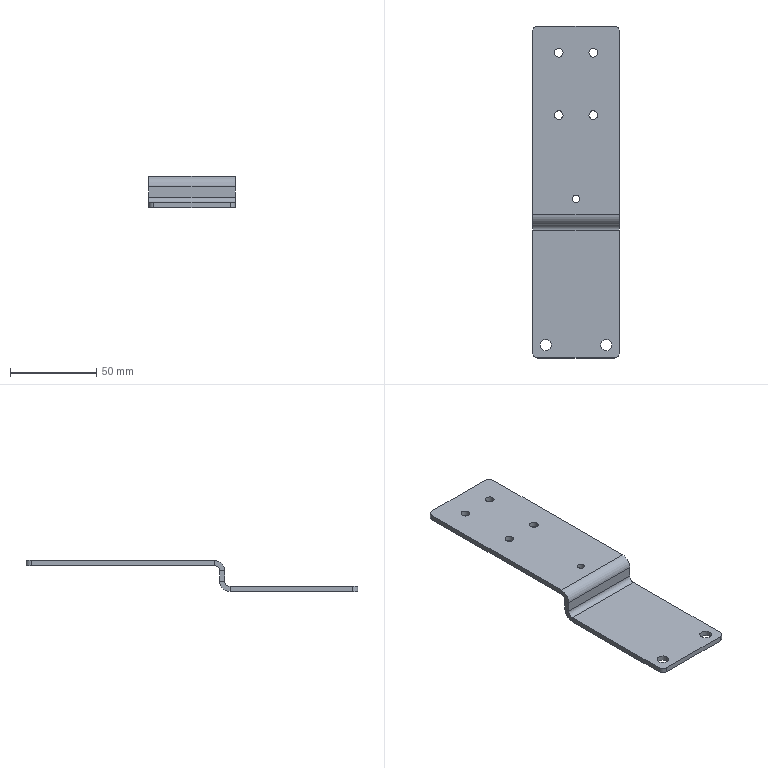Part | NX | 1 solid | 33 faces | box 50 x 192 x 18 mm | volume 29965 mm3 | plane 18 | cylinder 15 | commonest cylinder face diameters 6 x6 5 x4 6.6 x2 12 x2 4.2 x1
STEP:
#1=CARTESIAN_POINT('',(25.,40.,9.));
#2=VERTEX_POINT('',#1);
#3=CARTESIAN_POINT('',(25.,37.,9.));
#4=VERTEX_POINT('',#3);
#5=CARTESIAN_POINT('',(25.,40.,9.));
#6=DIRECTION('',(0.,-1.,0.));
#7=VECTOR('',#6,1000.);
#8=LINE('',#5,#7);
#9=EDGE_CURVE('',#2,#4,#8,.T.);
#10=ORIENTED_EDGE('',*,*,#9,.T.);
#11=CARTESIAN_POINT('',(25.,37.,3.));
#12=VERTEX_POINT('',#11);
#13=CARTESIAN_POINT('',(25.,37.,0.));
#14=DIRECTION('',(0.,0.,1.));
#15=VECTOR('',#14,1000.);
#16=LINE('',#13,#15);
#17=EDGE_CURVE('',#4,#12,#16,.F.);
#18=ORIENTED_EDGE('',*,*,#17,.T.);
#19=CARTESIAN_POINT('',(25.,40.,3.));
#20=VERTEX_POINT('',#19);
#21=CARTESIAN_POINT('',(25.,40.,3.));
#22=DIRECTION('',(0.,-1.,0.));
#23=VECTOR('',#22,1000.);
#24=LINE('',#21,#23);
#25=EDGE_CURVE('',#12,#20,#24,.F.);
#26=ORIENTED_EDGE('',*,*,#25,.T.);
#27=CARTESIAN_POINT('',(25.,40.,0.));
#28=DIRECTION('',(0.,0.,-1.));
#29=VECTOR('',#28,1000.);
#30=LINE('',#27,#29);
#31=EDGE_CURVE('',#2,#20,#30,.T.);
#32=ORIENTED_EDGE('',*,*,#31,.F.);
#33=EDGE_LOOP('',(#10,#18,#26,#32));
#34=FACE_BOUND('',#33,.T.);
#35=CARTESIAN_POINT('',(25.,40.,0.));
#36=DIRECTION('',(-1.,0.,0.));
#37=DIRECTION('',(0.,0.,1.));
#38=AXIS2_PLACEMENT_3D('',#35,#36,#37);
#39=PLANE('',#38);
#40=ADVANCED_FACE('',(#34),#39,.F.);
#41=CARTESIAN_POINT('',(-25.,40.,9.));
#42=VERTEX_POINT('',#41);
#43=CARTESIAN_POINT('',(-25.,37.,9.));
#44=VERTEX_POINT('',#43);
#45=CARTESIAN_POINT('',(-25.,40.,9.));
#46=DIRECTION('',(0.,-1.,0.));
#47=VECTOR('',#46,1000.);
#48=LINE('',#45,#47);
#49=EDGE_CURVE('',#42,#44,#48,.T.);
#50=ORIENTED_EDGE('',*,*,#49,.F.);
#51=CARTESIAN_POINT('',(-25.,40.,3.));
#52=VERTEX_POINT('',#51);
#53=CARTESIAN_POINT('',(-25.,40.,0.));
#54=DIRECTION('',(0.,0.,1.));
#55=VECTOR('',#54,1000.);
#56=LINE('',#53,#55);
#57=EDGE_CURVE('',#52,#42,#56,.T.);
#58=ORIENTED_EDGE('',*,*,#57,.F.);
#59=CARTESIAN_POINT('',(-25.,37.,3.));
#60=VERTEX_POINT('',#59);
#61=CARTESIAN_POINT('',(-25.,37.,3.));
#62=DIRECTION('',(0.,-1.,0.));
#63=VECTOR('',#62,1000.);
#64=LINE('',#61,#63);
#65=EDGE_CURVE('',#60,#52,#64,.F.);
#66=ORIENTED_EDGE('',*,*,#65,.F.);
#67=CARTESIAN_POINT('',(-25.,37.,15.));
#68=DIRECTION('',(0.,0.,-1.));
#69=VECTOR('',#68,1000.);
#70=LINE('',#67,#69);
#71=EDGE_CURVE('',#60,#44,#70,.F.);
#72=ORIENTED_EDGE('',*,*,#71,.T.);
#73=EDGE_LOOP('',(#50,#58,#66,#72));
#74=FACE_BOUND('',#73,.T.);
#75=CARTESIAN_POINT('',(-25.,40.,15.));
#76=DIRECTION('',(1.,0.,0.));
#77=DIRECTION('',(0.,0.,-1.));
#78=AXIS2_PLACEMENT_3D('',#75,#76,#77);
#79=PLANE('',#78);
#80=ADVANCED_FACE('',(#74),#79,.F.);
#81=CARTESIAN_POINT('',(25.,40.,9.));
#82=DIRECTION('',(1.,0.,0.));
#83=VECTOR('',#82,1000.);
#84=LINE('',#81,#83);
#85=EDGE_CURVE('',#2,#42,#84,.F.);
#86=ORIENTED_EDGE('',*,*,#85,.F.);
#87=ORIENTED_EDGE('',*,*,#31,.T.);
#88=CARTESIAN_POINT('',(25.,40.,3.));
#89=DIRECTION('',(-1.,0.,0.));
#90=VECTOR('',#89,1000.);
#91=LINE('',#88,#90);
#92=EDGE_CURVE('',#52,#20,#91,.F.);
#93=ORIENTED_EDGE('',*,*,#92,.F.);
#94=ORIENTED_EDGE('',*,*,#57,.T.);
#95=EDGE_LOOP('',(#86,#87,#93,#94));
#96=FACE_BOUND('',#95,.T.);
#97=CARTESIAN_POINT('',(0.,40.,0.));
#98=DIRECTION('',(0.,-1.,0.));
#99=DIRECTION('',(0.,0.,-1.));
#100=AXIS2_PLACEMENT_3D('',#97,#98,#99);
#101=PLANE('',#100);
#102=ADVANCED_FACE('',(#96),#101,.F.);
#103=ORIENTED_EDGE('',*,*,#17,.F.);
#104=CARTESIAN_POINT('',(25.,37.,9.));
#105=DIRECTION('',(1.,0.,0.));
#106=VECTOR('',#105,1000.);
#107=LINE('',#104,#106);
#108=EDGE_CURVE('',#4,#44,#107,.F.);
#109=ORIENTED_EDGE('',*,*,#108,.T.);
#110=ORIENTED_EDGE('',*,*,#71,.F.);
#111=CARTESIAN_POINT('',(25.,37.,3.));
#112=DIRECTION('',(-1.,0.,0.));
#113=VECTOR('',#112,1000.);
#114=LINE('',#111,#113);
#115=EDGE_CURVE('',#12,#60,#114,.T.);
#116=ORIENTED_EDGE('',*,*,#115,.F.);
#117=EDGE_LOOP('',(#103,#109,#110,#116));
#118=FACE_BOUND('',#117,.T.);
#119=CARTESIAN_POINT('',(0.,37.,0.));
#120=DIRECTION('',(0.,-1.,0.));
#121=DIRECTION('',(0.,0.,-1.));
#122=AXIS2_PLACEMENT_3D('',#119,#120,#121);
#123=PLANE('',#122);
#124=ADVANCED_FACE('',(#118),#123,.T.);
#125=CARTESIAN_POINT('',(-25.,34.,-3.));
#126=VERTEX_POINT('',#125);
#127=CARTESIAN_POINT('',(-25.,-37.,-3.));
#128=VERTEX_POINT('',#127);
#129=CARTESIAN_POINT('',(-25.,-40.,-3.));
#130=DIRECTION('',(0.,-1.,0.));
#131=VECTOR('',#130,1000.);
#132=LINE('',#129,#131);
#133=EDGE_CURVE('',#126,#128,#132,.T.);
#134=ORIENTED_EDGE('',*,*,#133,.T.);
#135=CARTESIAN_POINT('',(-25.,-37.,0.));
#136=VERTEX_POINT('',#135);
#137=CARTESIAN_POINT('',(-25.,-37.,-3.));
#138=DIRECTION('',(0.,0.,1.));
#139=VECTOR('',#138,1000.);
#140=LINE('',#137,#139);
#141=EDGE_CURVE('',#128,#136,#140,.T.);
#142=ORIENTED_EDGE('',*,*,#141,.T.);
#143=CARTESIAN_POINT('',(-25.,34.,0.));
#144=VERTEX_POINT('',#143);
#145=CARTESIAN_POINT('',(-25.,-40.,0.));
#146=DIRECTION('',(0.,-1.,0.));
#147=VECTOR('',#146,1000.);
#148=LINE('',#145,#147);
#149=EDGE_CURVE('',#144,#136,#148,.T.);
#150=ORIENTED_EDGE('',*,*,#149,.F.);
#151=CARTESIAN_POINT('',(-25.,34.,0.));
#152=DIRECTION('',(0.,0.,-1.));
#153=VECTOR('',#152,1000.);
#154=LINE('',#151,#153);
#155=EDGE_CURVE('',#144,#126,#154,.T.);
#156=ORIENTED_EDGE('',*,*,#155,.T.);
#157=EDGE_LOOP('',(#134,#142,#150,#156));
#158=FACE_BOUND('',#157,.T.);
#159=CARTESIAN_POINT('',(-25.,-40.,-3.));
#160=DIRECTION('',(-1.,0.,0.));
#161=DIRECTION('',(0.,0.,1.));
#162=AXIS2_PLACEMENT_3D('',#159,#160,#161);
#163=PLANE('',#162);
#164=ADVANCED_FACE('',(#158),#163,.T.);
#165=CARTESIAN_POINT('',(-14.2,-32.5,-3.));
#166=VERTEX_POINT('',#165);
#167=CARTESIAN_POINT('',(-17.5,-32.5,-3.));
#168=DIRECTION('',(0.,0.,1.));
#169=DIRECTION('',(1.,0.,0.));
#170=AXIS2_PLACEMENT_3D('',#167,#168,#169);
#171=CIRCLE('',#170,3.3);
#172=EDGE_CURVE('',#166,#166,#171,.T.);
#173=ORIENTED_EDGE('',*,*,#172,.T.);
#174=EDGE_LOOP('',(#173));
#175=FACE_BOUND('',#174,.T.);
#176=CARTESIAN_POINT('',(20.8,-32.5,-3.));
#177=VERTEX_POINT('',#176);
#178=CARTESIAN_POINT('',(17.5,-32.5,-3.));
#179=DIRECTION('',(0.,0.,1.));
#180=DIRECTION('',(1.,0.,0.));
#181=AXIS2_PLACEMENT_3D('',#178,#179,#180);
#182=CIRCLE('',#181,3.3);
#183=EDGE_CURVE('',#177,#177,#182,.T.);
#184=ORIENTED_EDGE('',*,*,#183,.T.);
#185=EDGE_LOOP('',(#184));
#186=FACE_BOUND('',#185,.T.);
#187=CARTESIAN_POINT('',(25.,-37.,-3.));
#188=VERTEX_POINT('',#187);
#189=CARTESIAN_POINT('',(25.,34.,-3.));
#190=VERTEX_POINT('',#189);
#191=CARTESIAN_POINT('',(25.,-40.,-3.));
#192=DIRECTION('',(0.,1.,0.));
#193=VECTOR('',#192,1000.);
#194=LINE('',#191,#193);
#195=EDGE_CURVE('',#188,#190,#194,.T.);
#196=ORIENTED_EDGE('',*,*,#195,.F.);
#197=CARTESIAN_POINT('',(22.,-40.,-3.));
#198=VERTEX_POINT('',#197);
#199=CARTESIAN_POINT('',(22.,-37.,-3.));
#200=DIRECTION('',(0.,0.,-1.));
#201=DIRECTION('',(-1.,0.,0.));
#202=AXIS2_PLACEMENT_3D('',#199,#200,#201);
#203=CIRCLE('',#202,3.);
#204=EDGE_CURVE('',#188,#198,#203,.T.);
#205=ORIENTED_EDGE('',*,*,#204,.T.);
#206=CARTESIAN_POINT('',(-22.,-40.,-3.));
#207=VERTEX_POINT('',#206);
#208=CARTESIAN_POINT('',(-25.,-40.,-3.));
#209=DIRECTION('',(1.,0.,0.));
#210=VECTOR('',#209,1000.);
#211=LINE('',#208,#210);
#212=EDGE_CURVE('',#207,#198,#211,.T.);
#213=ORIENTED_EDGE('',*,*,#212,.F.);
#214=CARTESIAN_POINT('',(-22.,-37.,-3.));
#215=DIRECTION('',(0.,0.,-1.));
#216=DIRECTION('',(-1.,0.,0.));
#217=AXIS2_PLACEMENT_3D('',#214,#215,#216);
#218=CIRCLE('',#217,3.);
#219=EDGE_CURVE('',#207,#128,#218,.T.);
#220=ORIENTED_EDGE('',*,*,#219,.T.);
#221=ORIENTED_EDGE('',*,*,#133,.F.);
#222=CARTESIAN_POINT('',(-25.,34.,-3.));
#223=DIRECTION('',(-1.,0.,0.));
#224=VECTOR('',#223,1000.);
#225=LINE('',#222,#224);
#226=EDGE_CURVE('',#126,#190,#225,.F.);
#227=ORIENTED_EDGE('',*,*,#226,.T.);
#228=EDGE_LOOP('',(#196,#205,#213,#220,#221,#227));
#229=FACE_BOUND('',#228,.T.);
#230=CARTESIAN_POINT('',(0.,0.,-3.));
#231=DIRECTION('',(0.,0.,-1.));
#232=DIRECTION('',(-1.,0.,0.));
#233=AXIS2_PLACEMENT_3D('',#230,#231,#232);
#234=PLANE('',#233);
#235=ADVANCED_FACE('',(#175,#186,#229),#234,.T.);
#236=CARTESIAN_POINT('',(-14.2,-32.5,0.));
#237=VERTEX_POINT('',#236);
#238=CARTESIAN_POINT('',(-17.5,-32.5,0.));
#239=DIRECTION('',(0.,0.,1.));
#240=DIRECTION('',(1.,0.,0.));
#241=AXIS2_PLACEMENT_3D('',#238,#239,#240);
#242=CIRCLE('',#241,3.3);
#243=EDGE_CURVE('',#237,#237,#242,.T.);
#244=ORIENTED_EDGE('',*,*,#243,.F.);
#245=EDGE_LOOP('',(#244));
#246=FACE_BOUND('',#245,.T.);
#247=CARTESIAN_POINT('',(20.8,-32.5,0.));
#248=VERTEX_POINT('',#247);
#249=CARTESIAN_POINT('',(17.5,-32.5,0.));
#250=DIRECTION('',(0.,0.,1.));
#251=DIRECTION('',(1.,0.,0.));
#252=AXIS2_PLACEMENT_3D('',#249,#250,#251);
#253=CIRCLE('',#252,3.3);
#254=EDGE_CURVE('',#248,#248,#253,.T.);
#255=ORIENTED_EDGE('',*,*,#254,.F.);
#256=EDGE_LOOP('',(#255));
#257=FACE_BOUND('',#256,.T.);
#258=CARTESIAN_POINT('',(-22.,-40.,0.));
#259=VERTEX_POINT('',#258);
#260=CARTESIAN_POINT('',(22.,-40.,0.));
#261=VERTEX_POINT('',#260);
#262=CARTESIAN_POINT('',(-25.,-40.,0.));
#263=DIRECTION('',(1.,0.,0.));
#264=VECTOR('',#263,1000.);
#265=LINE('',#262,#264);
#266=EDGE_CURVE('',#259,#261,#265,.T.);
#267=ORIENTED_EDGE('',*,*,#266,.T.);
#268=CARTESIAN_POINT('',(25.,-37.,0.));
#269=VERTEX_POINT('',#268);
#270=CARTESIAN_POINT('',(22.,-37.,0.));
#271=DIRECTION('',(0.,0.,-1.));
#272=DIRECTION('',(-1.,0.,0.));
#273=AXIS2_PLACEMENT_3D('',#270,#271,#272);
#274=CIRCLE('',#273,3.);
#275=EDGE_CURVE('',#261,#269,#274,.F.);
#276=ORIENTED_EDGE('',*,*,#275,.T.);
#277=CARTESIAN_POINT('',(25.,34.,0.));
#278=VERTEX_POINT('',#277);
#279=CARTESIAN_POINT('',(25.,-40.,0.));
#280=DIRECTION('',(0.,1.,0.));
#281=VECTOR('',#280,1000.);
#282=LINE('',#279,#281);
#283=EDGE_CURVE('',#269,#278,#282,.T.);
#284=ORIENTED_EDGE('',*,*,#283,.T.);
#285=CARTESIAN_POINT('',(-25.,34.,0.));
#286=DIRECTION('',(-1.,0.,0.));
#287=VECTOR('',#286,1000.);
#288=LINE('',#285,#287);
#289=EDGE_CURVE('',#144,#278,#288,.F.);
#290=ORIENTED_EDGE('',*,*,#289,.F.);
#291=ORIENTED_EDGE('',*,*,#149,.T.);
#292=CARTESIAN_POINT('',(-22.,-37.,0.));
#293=DIRECTION('',(0.,0.,-1.));
#294=DIRECTION('',(-1.,0.,0.));
#295=AXIS2_PLACEMENT_3D('',#292,#293,#294);
#296=CIRCLE('',#295,3.);
#297=EDGE_CURVE('',#136,#259,#296,.F.);
#298=ORIENTED_EDGE('',*,*,#297,.T.);
#299=EDGE_LOOP('',(#267,#276,#284,#290,#291,#298));
#300=FACE_BOUND('',#299,.T.);
#301=CARTESIAN_POINT('',(0.,0.,0.));
#302=DIRECTION('',(0.,0.,-1.));
#303=DIRECTION('',(-1.,0.,0.));
#304=AXIS2_PLACEMENT_3D('',#301,#302,#303);
#305=PLANE('',#304);
#306=ADVANCED_FACE('',(#246,#257,#300),#305,.F.);
#307=ORIENTED_EDGE('',*,*,#283,.F.);
#308=CARTESIAN_POINT('',(25.,-37.,-3.));
#309=DIRECTION('',(0.,0.,1.));
#310=VECTOR('',#309,1000.);
#311=LINE('',#308,#310);
#312=EDGE_CURVE('',#269,#188,#311,.F.);
#313=ORIENTED_EDGE('',*,*,#312,.T.);
#314=ORIENTED_EDGE('',*,*,#195,.T.);
#315=CARTESIAN_POINT('',(25.,34.,0.));
#316=DIRECTION('',(0.,0.,-1.));
#317=VECTOR('',#316,1000.);
#318=LINE('',#315,#317);
#319=EDGE_CURVE('',#278,#190,#318,.T.);
#320=ORIENTED_EDGE('',*,*,#319,.F.);
#321=EDGE_LOOP('',(#307,#313,#314,#320));
#322=FACE_BOUND('',#321,.T.);
#323=CARTESIAN_POINT('',(25.,-40.,-3.));
#324=DIRECTION('',(1.,0.,0.));
#325=DIRECTION('',(0.,0.,-1.));
#326=AXIS2_PLACEMENT_3D('',#323,#324,#325);
#327=PLANE('',#326);
#328=ADVANCED_FACE('',(#322),#327,.T.);
#329=ORIENTED_EDGE('',*,*,#212,.T.);
#330=CARTESIAN_POINT('',(22.,-40.,-3.));
#331=DIRECTION('',(0.,0.,1.));
#332=VECTOR('',#331,1000.);
#333=LINE('',#330,#332);
#334=EDGE_CURVE('',#198,#261,#333,.T.);
#335=ORIENTED_EDGE('',*,*,#334,.T.);
#336=ORIENTED_EDGE('',*,*,#266,.F.);
#337=CARTESIAN_POINT('',(-22.,-40.,-3.));
#338=DIRECTION('',(0.,0.,1.));
#339=VECTOR('',#338,1000.);
#340=LINE('',#337,#339);
#341=EDGE_CURVE('',#259,#207,#340,.F.);
#342=ORIENTED_EDGE('',*,*,#341,.T.);
#343=EDGE_LOOP('',(#329,#335,#336,#342));
#344=FACE_BOUND('',#343,.T.);
#345=CARTESIAN_POINT('',(-25.,-40.,-3.));
#346=DIRECTION('',(0.,-1.,0.));
#347=DIRECTION('',(0.,0.,-1.));
#348=AXIS2_PLACEMENT_3D('',#345,#346,#347);
#349=PLANE('',#348);
#350=ADVANCED_FACE('',(#344),#349,.T.);
#351=ORIENTED_EDGE('',*,*,#25,.F.);
#352=CARTESIAN_POINT('',(25.,34.,3.));
#353=DIRECTION('',(-1.,0.,0.));
#354=DIRECTION('',(0.,0.,1.));
#355=AXIS2_PLACEMENT_3D('',#352,#353,#354);
#356=CIRCLE('',#355,3.);
#357=EDGE_CURVE('',#278,#12,#356,.F.);
#358=ORIENTED_EDGE('',*,*,#357,.F.);
#359=ORIENTED_EDGE('',*,*,#319,.T.);
#360=CARTESIAN_POINT('',(25.,34.,3.));
#361=DIRECTION('',(-1.,0.,0.));
#362=DIRECTION('',(0.,0.,1.));
#363=AXIS2_PLACEMENT_3D('',#360,#361,#362);
#364=CIRCLE('',#363,6.);
#365=EDGE_CURVE('',#190,#20,#364,.F.);
#366=ORIENTED_EDGE('',*,*,#365,.T.);
#367=EDGE_LOOP('',(#351,#358,#359,#366));
#368=FACE_BOUND('',#367,.T.);
#369=CARTESIAN_POINT('',(25.,34.,3.));
#370=DIRECTION('',(1.,0.,0.));
#371=DIRECTION('',(0.,0.,-1.));
#372=AXIS2_PLACEMENT_3D('',#369,#370,#371);
#373=PLANE('',#372);
#374=ADVANCED_FACE('',(#368),#373,.T.);
#375=CARTESIAN_POINT('',(-25.,34.,3.));
#376=DIRECTION('',(-1.,0.,0.));
#377=DIRECTION('',(0.,0.,1.));
#378=AXIS2_PLACEMENT_3D('',#375,#376,#377);
#379=CIRCLE('',#378,3.);
#380=EDGE_CURVE('',#60,#144,#379,.T.);
#381=ORIENTED_EDGE('',*,*,#380,.F.);
#382=ORIENTED_EDGE('',*,*,#65,.T.);
#383=CARTESIAN_POINT('',(-25.,34.,3.));
#384=DIRECTION('',(-1.,0.,0.));
#385=DIRECTION('',(0.,0.,1.));
#386=AXIS2_PLACEMENT_3D('',#383,#384,#385);
#387=CIRCLE('',#386,6.);
#388=EDGE_CURVE('',#52,#126,#387,.T.);
#389=ORIENTED_EDGE('',*,*,#388,.T.);
#390=ORIENTED_EDGE('',*,*,#155,.F.);
#391=EDGE_LOOP('',(#381,#382,#389,#390));
#392=FACE_BOUND('',#391,.T.);
#393=CARTESIAN_POINT('',(-25.,34.,3.));
#394=DIRECTION('',(1.,0.,0.));
#395=DIRECTION('',(0.,0.,-1.));
#396=AXIS2_PLACEMENT_3D('',#393,#394,#395);
#397=PLANE('',#396);
#398=ADVANCED_FACE('',(#392),#397,.F.);
#399=ORIENTED_EDGE('',*,*,#226,.F.);
#400=ORIENTED_EDGE('',*,*,#388,.F.);
#401=ORIENTED_EDGE('',*,*,#92,.T.);
#402=ORIENTED_EDGE('',*,*,#365,.F.);
#403=EDGE_LOOP('',(#399,#400,#401,#402));
#404=FACE_BOUND('',#403,.T.);
#405=CARTESIAN_POINT('',(-25.,34.,3.));
#406=DIRECTION('',(-1.,0.,0.));
#407=DIRECTION('',(0.,1.,0.));
#408=AXIS2_PLACEMENT_3D('',#405,#406,#407);
#409=CYLINDRICAL_SURFACE('',#408,6.);
#410=ADVANCED_FACE('',(#404),#409,.T.);
#411=ORIENTED_EDGE('',*,*,#289,.T.);
#412=ORIENTED_EDGE('',*,*,#357,.T.);
#413=ORIENTED_EDGE('',*,*,#115,.T.);
#414=ORIENTED_EDGE('',*,*,#380,.T.);
#415=EDGE_LOOP('',(#411,#412,#413,#414));
#416=FACE_BOUND('',#415,.T.);
#417=CARTESIAN_POINT('',(-25.,34.,3.));
#418=DIRECTION('',(-1.,0.,0.));
#419=DIRECTION('',(0.,1.,0.));
#420=AXIS2_PLACEMENT_3D('',#417,#418,#419);
#421=CYLINDRICAL_SURFACE('',#420,3.);
#422=ADVANCED_FACE('',(#416),#421,.F.);
#423=CARTESIAN_POINT('',(-25.,43.,12.));
#424=VERTEX_POINT('',#423);
#425=CARTESIAN_POINT('',(-25.,43.,15.));
#426=VERTEX_POINT('',#425);
#427=CARTESIAN_POINT('',(-25.,43.,15.));
#428=DIRECTION('',(0.,0.,-1.));
#429=VECTOR('',#428,1000.);
#430=LINE('',#427,#429);
#431=EDGE_CURVE('',#424,#426,#430,.F.);
#432=ORIENTED_EDGE('',*,*,#431,.F.);
#433=CARTESIAN_POINT('',(-25.,43.,9.));
#434=DIRECTION('',(1.,0.,0.));
#435=DIRECTION('',(0.,0.,-1.));
#436=AXIS2_PLACEMENT_3D('',#433,#434,#435);
#437=CIRCLE('',#436,3.);
#438=EDGE_CURVE('',#42,#424,#437,.F.);
#439=ORIENTED_EDGE('',*,*,#438,.F.);
#440=ORIENTED_EDGE('',*,*,#49,.T.);
#441=CARTESIAN_POINT('',(-25.,43.,9.));
#442=DIRECTION('',(1.,0.,0.));
#443=DIRECTION('',(0.,0.,-1.));
#444=AXIS2_PLACEMENT_3D('',#441,#442,#443);
#445=CIRCLE('',#444,6.);
#446=EDGE_CURVE('',#44,#426,#445,.F.);
#447=ORIENTED_EDGE('',*,*,#446,.T.);
#448=EDGE_LOOP('',(#432,#439,#440,#447));
#449=FACE_BOUND('',#448,.T.);
#450=CARTESIAN_POINT('',(-25.,43.,9.));
#451=DIRECTION('',(-1.,0.,0.));
#452=DIRECTION('',(0.,0.,1.));
#453=AXIS2_PLACEMENT_3D('',#450,#451,#452);
#454=PLANE('',#453);
#455=ADVANCED_FACE('',(#449),#454,.T.);
#456=CARTESIAN_POINT('',(25.,43.,12.));
#457=VERTEX_POINT('',#456);
#458=CARTESIAN_POINT('',(25.,43.,9.));
#459=DIRECTION('',(1.,0.,0.));
#460=DIRECTION('',(0.,0.,-1.));
#461=AXIS2_PLACEMENT_3D('',#458,#459,#460);
#462=CIRCLE('',#461,3.);
#463=EDGE_CURVE('',#457,#2,#462,.T.);
#464=ORIENTED_EDGE('',*,*,#463,.F.);
#465=CARTESIAN_POINT('',(25.,43.,15.));
#466=VERTEX_POINT('',#465);
#467=CARTESIAN_POINT('',(25.,43.,12.));
#468=DIRECTION('',(0.,0.,-1.));
#469=VECTOR('',#468,1000.);
#470=LINE('',#467,#469);
#471=EDGE_CURVE('',#457,#466,#470,.F.);
#472=ORIENTED_EDGE('',*,*,#471,.T.);
#473=CARTESIAN_POINT('',(25.,43.,9.));
#474=DIRECTION('',(1.,0.,0.));
#475=DIRECTION('',(0.,0.,-1.));
#476=AXIS2_PLACEMENT_3D('',#473,#474,#475);
#477=CIRCLE('',#476,6.);
#478=EDGE_CURVE('',#466,#4,#477,.T.);
#479=ORIENTED_EDGE('',*,*,#478,.T.);
#480=ORIENTED_EDGE('',*,*,#9,.F.);
#481=EDGE_LOOP('',(#464,#472,#479,#480));
#482=FACE_BOUND('',#481,.T.);
#483=CARTESIAN_POINT('',(25.,43.,9.));
#484=DIRECTION('',(-1.,0.,0.));
#485=DIRECTION('',(0.,0.,1.));
#486=AXIS2_PLACEMENT_3D('',#483,#484,#485);
#487=PLANE('',#486);
#488=ADVANCED_FACE('',(#482),#487,.F.);
#489=ORIENTED_EDGE('',*,*,#108,.F.);
#490=ORIENTED_EDGE('',*,*,#478,.F.);
#491=CARTESIAN_POINT('',(-25.,43.,15.));
#492=DIRECTION('',(1.,0.,0.));
#493=VECTOR('',#492,1000.);
#494=LINE('',#491,#493);
#495=EDGE_CURVE('',#466,#426,#494,.F.);
#496=ORIENTED_EDGE('',*,*,#495,.T.);
#497=ORIENTED_EDGE('',*,*,#446,.F.);
#498=EDGE_LOOP('',(#489,#490,#496,#497));
#499=FACE_BOUND('',#498,.T.);
#500=CARTESIAN_POINT('',(25.,43.,9.));
#501=DIRECTION('',(1.,0.,0.));
#502=DIRECTION('',(0.,0.,1.));
#503=AXIS2_PLACEMENT_3D('',#500,#501,#502);
#504=CYLINDRICAL_SURFACE('',#503,6.);
#505=ADVANCED_FACE('',(#499),#504,.T.);
#506=ORIENTED_EDGE('',*,*,#85,.T.);
#507=ORIENTED_EDGE('',*,*,#438,.T.);
#508=CARTESIAN_POINT('',(-25.,43.,12.));
#509=DIRECTION('',(1.,0.,0.));
#510=VECTOR('',#509,1000.);
#511=LINE('',#508,#510);
#512=EDGE_CURVE('',#424,#457,#511,.T.);
#513=ORIENTED_EDGE('',*,*,#512,.T.);
#514=ORIENTED_EDGE('',*,*,#463,.T.);
#515=EDGE_LOOP('',(#506,#507,#513,#514));
#516=FACE_BOUND('',#515,.T.);
#517=CARTESIAN_POINT('',(25.,43.,9.));
#518=DIRECTION('',(1.,0.,0.));
#519=DIRECTION('',(0.,0.,1.));
#520=AXIS2_PLACEMENT_3D('',#517,#518,#519);
#521=CYLINDRICAL_SURFACE('',#520,3.);
#522=ADVANCED_FACE('',(#516),#521,.F.);
#523=CARTESIAN_POINT('',(-25.,149.,15.));
#524=VERTEX_POINT('',#523);
#525=CARTESIAN_POINT('',(-25.,0.,15.));
#526=DIRECTION('',(0.,-1.,0.));
#527=VECTOR('',#526,1000.);
#528=LINE('',#525,#527);
#529=EDGE_CURVE('',#524,#426,#528,.T.);
#530=ORIENTED_EDGE('',*,*,#529,.F.);
#531=CARTESIAN_POINT('',(-25.,149.,12.));
#532=VERTEX_POINT('',#531);
#533=CARTESIAN_POINT('',(-25.,149.,15.));
#534=DIRECTION('',(0.,0.,-1.));
#535=VECTOR('',#534,1000.);
#536=LINE('',#533,#535);
#537=EDGE_CURVE('',#524,#532,#536,.T.);
#538=ORIENTED_EDGE('',*,*,#537,.T.);
#539=CARTESIAN_POINT('',(-25.,40.,12.));
#540=DIRECTION('',(0.,1.,0.));
#541=VECTOR('',#540,1000.);
#542=LINE('',#539,#541);
#543=EDGE_CURVE('',#532,#424,#542,.F.);
#544=ORIENTED_EDGE('',*,*,#543,.T.);
#545=ORIENTED_EDGE('',*,*,#431,.T.);
#546=EDGE_LOOP('',(#530,#538,#544,#545));
#547=FACE_BOUND('',#546,.T.);
#548=CARTESIAN_POINT('',(-25.,40.,15.));
#549=DIRECTION('',(1.,0.,0.));
#550=DIRECTION('',(0.,0.,-1.));
#551=AXIS2_PLACEMENT_3D('',#548,#549,#550);
#552=PLANE('',#551);
#553=ADVANCED_FACE('',(#547),#552,.F.);
#554=CARTESIAN_POINT('',(25.,149.,12.));
#555=VERTEX_POINT('',#554);
#556=CARTESIAN_POINT('',(25.,152.,12.));
#557=DIRECTION('',(0.,-1.,0.));
#558=VECTOR('',#557,1000.);
#559=LINE('',#556,#558);
#560=EDGE_CURVE('',#457,#555,#559,.F.);
#561=ORIENTED_EDGE('',*,*,#560,.T.);
#562=CARTESIAN_POINT('',(25.,149.,15.));
#563=VERTEX_POINT('',#562);
#564=CARTESIAN_POINT('',(25.,149.,15.));
#565=DIRECTION('',(0.,0.,-1.));
#566=VECTOR('',#565,1000.);
#567=LINE('',#564,#566);
#568=EDGE_CURVE('',#555,#563,#567,.F.);
#569=ORIENTED_EDGE('',*,*,#568,.T.);
#570=CARTESIAN_POINT('',(25.,0.,15.));
#571=DIRECTION('',(0.,1.,0.));
#572=VECTOR('',#571,1000.);
#573=LINE('',#570,#572);
#574=EDGE_CURVE('',#466,#563,#573,.T.);
#575=ORIENTED_EDGE('',*,*,#574,.F.);
#576=ORIENTED_EDGE('',*,*,#471,.F.);
#577=EDGE_LOOP('',(#561,#569,#575,#576));
#578=FACE_BOUND('',#577,.T.);
#579=CARTESIAN_POINT('',(25.,152.,15.));
#580=DIRECTION('',(-1.,0.,0.));
#581=DIRECTION('',(0.,-1.,0.));
#582=AXIS2_PLACEMENT_3D('',#579,#580,#581);
#583=PLANE('',#582);
#584=ADVANCED_FACE('',(#578),#583,.F.);
#585=CARTESIAN_POINT('',(2.1,52.,15.));
#586=VERTEX_POINT('',#585);
#587=CARTESIAN_POINT('',(0.,52.,15.));
#588=DIRECTION('',(0.,0.,1.));
#589=DIRECTION('',(1.,0.,0.));
#590=AXIS2_PLACEMENT_3D('',#587,#588,#589);
#591=CIRCLE('',#590,2.1);
#592=EDGE_CURVE('',#586,#586,#591,.T.);
#593=ORIENTED_EDGE('',*,*,#592,.F.);
#594=EDGE_LOOP('',(#593));
#595=FACE_BOUND('',#594,.T.);
#596=CARTESIAN_POINT('',(12.5,136.5,15.));
#597=VERTEX_POINT('',#596);
#598=CARTESIAN_POINT('',(10.,136.5,15.));
#599=DIRECTION('',(0.,0.,1.));
#600=DIRECTION('',(1.,0.,0.));
#601=AXIS2_PLACEMENT_3D('',#598,#599,#600);
#602=CIRCLE('',#601,2.5);
#603=EDGE_CURVE('',#597,#597,#602,.T.);
#604=ORIENTED_EDGE('',*,*,#603,.F.);
#605=EDGE_LOOP('',(#604));
#606=FACE_BOUND('',#605,.T.);
#607=CARTESIAN_POINT('',(-7.5,136.5,15.));
#608=VERTEX_POINT('',#607);
#609=CARTESIAN_POINT('',(-10.,136.5,15.));
#610=DIRECTION('',(0.,0.,1.));
#611=DIRECTION('',(1.,0.,0.));
#612=AXIS2_PLACEMENT_3D('',#609,#610,#611);
#613=CIRCLE('',#612,2.5);
#614=EDGE_CURVE('',#608,#608,#613,.T.);
#615=ORIENTED_EDGE('',*,*,#614,.F.);
#616=EDGE_LOOP('',(#615));
#617=FACE_BOUND('',#616,.T.);
#618=CARTESIAN_POINT('',(-7.5,100.5,15.));
#619=VERTEX_POINT('',#618);
#620=CARTESIAN_POINT('',(-10.,100.5,15.));
#621=DIRECTION('',(0.,0.,1.));
#622=DIRECTION('',(1.,0.,0.));
#623=AXIS2_PLACEMENT_3D('',#620,#621,#622);
#624=CIRCLE('',#623,2.5);
#625=EDGE_CURVE('',#619,#619,#624,.T.);
#626=ORIENTED_EDGE('',*,*,#625,.F.);
#627=EDGE_LOOP('',(#626));
#628=FACE_BOUND('',#627,.T.);
#629=CARTESIAN_POINT('',(12.5,100.5,15.));
#630=VERTEX_POINT('',#629);
#631=CARTESIAN_POINT('',(10.,100.5,15.));
#632=DIRECTION('',(0.,0.,1.));
#633=DIRECTION('',(1.,0.,0.));
#634=AXIS2_PLACEMENT_3D('',#631,#632,#633);
#635=CIRCLE('',#634,2.5);
#636=EDGE_CURVE('',#630,#630,#635,.T.);
#637=ORIENTED_EDGE('',*,*,#636,.F.);
#638=EDGE_LOOP('',(#637));
#639=FACE_BOUND('',#638,.T.);
#640=ORIENTED_EDGE('',*,*,#574,.T.);
#641=CARTESIAN_POINT('',(22.,152.,15.));
#642=VERTEX_POINT('',#641);
#643=CARTESIAN_POINT('',(22.,149.,15.));
#644=DIRECTION('',(0.,0.,-1.));
#645=DIRECTION('',(-1.,0.,0.));
#646=AXIS2_PLACEMENT_3D('',#643,#644,#645);
#647=CIRCLE('',#646,3.);
#648=EDGE_CURVE('',#563,#642,#647,.F.);
#649=ORIENTED_EDGE('',*,*,#648,.T.);
#650=CARTESIAN_POINT('',(-22.,152.,15.));
#651=VERTEX_POINT('',#650);
#652=CARTESIAN_POINT('',(0.,152.,15.));
#653=DIRECTION('',(-1.,0.,0.));
#654=VECTOR('',#653,1000.);
#655=LINE('',#652,#654);
#656=EDGE_CURVE('',#642,#651,#655,.T.);
#657=ORIENTED_EDGE('',*,*,#656,.T.);
#658=CARTESIAN_POINT('',(-22.,149.,15.));
#659=DIRECTION('',(0.,0.,-1.));
#660=DIRECTION('',(-1.,0.,0.));
#661=AXIS2_PLACEMENT_3D('',#658,#659,#660);
#662=CIRCLE('',#661,3.);
#663=EDGE_CURVE('',#651,#524,#662,.F.);
#664=ORIENTED_EDGE('',*,*,#663,.T.);
#665=ORIENTED_EDGE('',*,*,#529,.T.);
#666=ORIENTED_EDGE('',*,*,#495,.F.);
#667=EDGE_LOOP('',(#640,#649,#657,#664,#665,#666));
#668=FACE_BOUND('',#667,.T.);
#669=CARTESIAN_POINT('',(0.,0.,15.));
#670=DIRECTION('',(0.,0.,-1.));
#671=DIRECTION('',(-1.,0.,0.));
#672=AXIS2_PLACEMENT_3D('',#669,#670,#671);
#673=PLANE('',#672);
#674=ADVANCED_FACE('',(#595,#606,#617,#628,#639,#668),#673,.F.);
#675=CARTESIAN_POINT('',(-2.1,52.,12.));
#676=VERTEX_POINT('',#675);
#677=CARTESIAN_POINT('',(0.,52.,12.));
#678=DIRECTION('',(0.,0.,-1.));
#679=DIRECTION('',(-1.,0.,0.));
#680=AXIS2_PLACEMENT_3D('',#677,#678,#679);
#681=CIRCLE('',#680,2.1);
#682=EDGE_CURVE('',#676,#676,#681,.T.);
#683=ORIENTED_EDGE('',*,*,#682,.F.);
#684=EDGE_LOOP('',(#683));
#685=FACE_BOUND('',#684,.T.);
#686=CARTESIAN_POINT('',(7.5,136.5,12.));
#687=VERTEX_POINT('',#686);
#688=CARTESIAN_POINT('',(10.,136.5,12.));
#689=DIRECTION('',(0.,0.,-1.));
#690=DIRECTION('',(-1.,0.,0.));
#691=AXIS2_PLACEMENT_3D('',#688,#689,#690);
#692=CIRCLE('',#691,2.5);
#693=EDGE_CURVE('',#687,#687,#692,.T.);
#694=ORIENTED_EDGE('',*,*,#693,.F.);
#695=EDGE_LOOP('',(#694));
#696=FACE_BOUND('',#695,.T.);
#697=CARTESIAN_POINT('',(-12.5,136.5,12.));
#698=VERTEX_POINT('',#697);
#699=CARTESIAN_POINT('',(-10.,136.5,12.));
#700=DIRECTION('',(0.,0.,-1.));
#701=DIRECTION('',(-1.,0.,0.));
#702=AXIS2_PLACEMENT_3D('',#699,#700,#701);
#703=CIRCLE('',#702,2.5);
#704=EDGE_CURVE('',#698,#698,#703,.T.);
#705=ORIENTED_EDGE('',*,*,#704,.F.);
#706=EDGE_LOOP('',(#705));
#707=FACE_BOUND('',#706,.T.);
#708=CARTESIAN_POINT('',(-12.5,100.5,12.));
#709=VERTEX_POINT('',#708);
#710=CARTESIAN_POINT('',(-10.,100.5,12.));
#711=DIRECTION('',(0.,0.,-1.));
#712=DIRECTION('',(-1.,0.,0.));
#713=AXIS2_PLACEMENT_3D('',#710,#711,#712);
#714=CIRCLE('',#713,2.5);
#715=EDGE_CURVE('',#709,#709,#714,.T.);
#716=ORIENTED_EDGE('',*,*,#715,.F.);
#717=EDGE_LOOP('',(#716));
#718=FACE_BOUND('',#717,.T.);
#719=CARTESIAN_POINT('',(7.5,100.5,12.));
#720=VERTEX_POINT('',#719);
#721=CARTESIAN_POINT('',(10.,100.5,12.));
#722=DIRECTION('',(0.,0.,-1.));
#723=DIRECTION('',(-1.,0.,0.));
#724=AXIS2_PLACEMENT_3D('',#721,#722,#723);
#725=CIRCLE('',#724,2.5);
#726=EDGE_CURVE('',#720,#720,#725,.T.);
#727=ORIENTED_EDGE('',*,*,#726,.F.);
#728=EDGE_LOOP('',(#727));
#729=FACE_BOUND('',#728,.T.);
#730=CARTESIAN_POINT('',(22.,152.,12.));
#731=VERTEX_POINT('',#730);
#732=CARTESIAN_POINT('',(-22.,152.,12.));
#733=VERTEX_POINT('',#732);
#734=CARTESIAN_POINT('',(-25.,152.,12.));
#735=DIRECTION('',(1.,0.,0.));
#736=VECTOR('',#735,1000.);
#737=LINE('',#734,#736);
#738=EDGE_CURVE('',#731,#733,#737,.F.);
#739=ORIENTED_EDGE('',*,*,#738,.F.);
#740=CARTESIAN_POINT('',(22.,149.,12.));
#741=DIRECTION('',(0.,0.,-1.));
#742=DIRECTION('',(-1.,0.,0.));
#743=AXIS2_PLACEMENT_3D('',#740,#741,#742);
#744=CIRCLE('',#743,3.);
#745=EDGE_CURVE('',#731,#555,#744,.T.);
#746=ORIENTED_EDGE('',*,*,#745,.T.);
#747=ORIENTED_EDGE('',*,*,#560,.F.);
#748=ORIENTED_EDGE('',*,*,#512,.F.);
#749=ORIENTED_EDGE('',*,*,#543,.F.);
#750=CARTESIAN_POINT('',(-22.,149.,12.));
#751=DIRECTION('',(0.,0.,-1.));
#752=DIRECTION('',(-1.,0.,0.));
#753=AXIS2_PLACEMENT_3D('',#750,#751,#752);
#754=CIRCLE('',#753,3.);
#755=EDGE_CURVE('',#532,#733,#754,.T.);
#756=ORIENTED_EDGE('',*,*,#755,.T.);
#757=EDGE_LOOP('',(#739,#746,#747,#748,#749,#756));
#758=FACE_BOUND('',#757,.T.);
#759=CARTESIAN_POINT('',(0.,0.,12.));
#760=DIRECTION('',(0.,0.,-1.));
#761=DIRECTION('',(-1.,0.,0.));
#762=AXIS2_PLACEMENT_3D('',#759,#760,#761);
#763=PLANE('',#762);
#764=ADVANCED_FACE('',(#685,#696,#707,#718,#729,#758),#763,.T.);
#765=ORIENTED_EDGE('',*,*,#656,.F.);
#766=CARTESIAN_POINT('',(22.,152.,15.));
#767=DIRECTION('',(0.,0.,-1.));
#768=VECTOR('',#767,1000.);
#769=LINE('',#766,#768);
#770=EDGE_CURVE('',#642,#731,#769,.T.);
#771=ORIENTED_EDGE('',*,*,#770,.T.);
#772=ORIENTED_EDGE('',*,*,#738,.T.);
#773=CARTESIAN_POINT('',(-22.,152.,15.));
#774=DIRECTION('',(0.,0.,-1.));
#775=VECTOR('',#774,1000.);
#776=LINE('',#773,#775);
#777=EDGE_CURVE('',#733,#651,#776,.F.);
#778=ORIENTED_EDGE('',*,*,#777,.T.);
#779=EDGE_LOOP('',(#765,#771,#772,#778));
#780=FACE_BOUND('',#779,.T.);
#781=CARTESIAN_POINT('',(-25.,152.,15.));
#782=DIRECTION('',(0.,-1.,0.));
#783=DIRECTION('',(0.,0.,-1.));
#784=AXIS2_PLACEMENT_3D('',#781,#782,#783);
#785=PLANE('',#784);
#786=ADVANCED_FACE('',(#780),#785,.F.);
#787=ORIENTED_EDGE('',*,*,#183,.F.);
#788=EDGE_LOOP('',(#787));
#789=FACE_BOUND('',#788,.T.);
#790=ORIENTED_EDGE('',*,*,#254,.T.);
#791=EDGE_LOOP('',(#790));
#792=FACE_BOUND('',#791,.T.);
#793=CARTESIAN_POINT('',(17.5,-32.5,0.));
#794=DIRECTION('',(0.,0.,1.));
#795=DIRECTION('',(1.,0.,0.));
#796=AXIS2_PLACEMENT_3D('',#793,#794,#795);
#797=CYLINDRICAL_SURFACE('',#796,3.3);
#798=ADVANCED_FACE('',(#789,#792),#797,.F.);
#799=ORIENTED_EDGE('',*,*,#172,.F.);
#800=EDGE_LOOP('',(#799));
#801=FACE_BOUND('',#800,.T.);
#802=ORIENTED_EDGE('',*,*,#243,.T.);
#803=EDGE_LOOP('',(#802));
#804=FACE_BOUND('',#803,.T.);
#805=CARTESIAN_POINT('',(-17.5,-32.5,0.));
#806=DIRECTION('',(0.,0.,1.));
#807=DIRECTION('',(1.,0.,0.));
#808=AXIS2_PLACEMENT_3D('',#805,#806,#807);
#809=CYLINDRICAL_SURFACE('',#808,3.3);
#810=ADVANCED_FACE('',(#801,#804),#809,.F.);
#811=ORIENTED_EDGE('',*,*,#726,.T.);
#812=EDGE_LOOP('',(#811));
#813=FACE_BOUND('',#812,.T.);
#814=ORIENTED_EDGE('',*,*,#636,.T.);
#815=EDGE_LOOP('',(#814));
#816=FACE_BOUND('',#815,.T.);
#817=CARTESIAN_POINT('',(10.,100.5,15.));
#818=DIRECTION('',(0.,0.,1.));
#819=DIRECTION('',(1.,0.,0.));
#820=AXIS2_PLACEMENT_3D('',#817,#818,#819);
#821=CYLINDRICAL_SURFACE('',#820,2.5);
#822=ADVANCED_FACE('',(#813,#816),#821,.F.);
#823=ORIENTED_EDGE('',*,*,#715,.T.);
#824=EDGE_LOOP('',(#823));
#825=FACE_BOUND('',#824,.T.);
#826=ORIENTED_EDGE('',*,*,#625,.T.);
#827=EDGE_LOOP('',(#826));
#828=FACE_BOUND('',#827,.T.);
#829=CARTESIAN_POINT('',(-10.,100.5,15.));
#830=DIRECTION('',(0.,0.,1.));
#831=DIRECTION('',(1.,0.,0.));
#832=AXIS2_PLACEMENT_3D('',#829,#830,#831);
#833=CYLINDRICAL_SURFACE('',#832,2.5);
#834=ADVANCED_FACE('',(#825,#828),#833,.F.);
#835=ORIENTED_EDGE('',*,*,#704,.T.);
#836=EDGE_LOOP('',(#835));
#837=FACE_BOUND('',#836,.T.);
#838=ORIENTED_EDGE('',*,*,#614,.T.);
#839=EDGE_LOOP('',(#838));
#840=FACE_BOUND('',#839,.T.);
#841=CARTESIAN_POINT('',(-10.,136.5,15.));
#842=DIRECTION('',(0.,0.,1.));
#843=DIRECTION('',(1.,0.,0.));
#844=AXIS2_PLACEMENT_3D('',#841,#842,#843);
#845=CYLINDRICAL_SURFACE('',#844,2.5);
#846=ADVANCED_FACE('',(#837,#840),#845,.F.);
#847=ORIENTED_EDGE('',*,*,#693,.T.);
#848=EDGE_LOOP('',(#847));
#849=FACE_BOUND('',#848,.T.);
#850=ORIENTED_EDGE('',*,*,#603,.T.);
#851=EDGE_LOOP('',(#850));
#852=FACE_BOUND('',#851,.T.);
#853=CARTESIAN_POINT('',(10.,136.5,15.));
#854=DIRECTION('',(0.,0.,1.));
#855=DIRECTION('',(1.,0.,0.));
#856=AXIS2_PLACEMENT_3D('',#853,#854,#855);
#857=CYLINDRICAL_SURFACE('',#856,2.5);
#858=ADVANCED_FACE('',(#849,#852),#857,.F.);
#859=ORIENTED_EDGE('',*,*,#682,.T.);
#860=EDGE_LOOP('',(#859));
#861=FACE_BOUND('',#860,.T.);
#862=ORIENTED_EDGE('',*,*,#592,.T.);
#863=EDGE_LOOP('',(#862));
#864=FACE_BOUND('',#863,.T.);
#865=CARTESIAN_POINT('',(0.,52.,15.));
#866=DIRECTION('',(0.,0.,1.));
#867=DIRECTION('',(1.,0.,0.));
#868=AXIS2_PLACEMENT_3D('',#865,#866,#867);
#869=CYLINDRICAL_SURFACE('',#868,2.1);
#870=ADVANCED_FACE('',(#861,#864),#869,.F.);
#871=ORIENTED_EDGE('',*,*,#648,.F.);
#872=ORIENTED_EDGE('',*,*,#568,.F.);
#873=ORIENTED_EDGE('',*,*,#745,.F.);
#874=ORIENTED_EDGE('',*,*,#770,.F.);
#875=EDGE_LOOP('',(#871,#872,#873,#874));
#876=FACE_BOUND('',#875,.T.);
#877=CARTESIAN_POINT('',(22.,149.,15.));
#878=DIRECTION('',(0.,0.,-1.));
#879=DIRECTION('',(-1.,0.,0.));
#880=AXIS2_PLACEMENT_3D('',#877,#878,#879);
#881=CYLINDRICAL_SURFACE('',#880,3.);
#882=ADVANCED_FACE('',(#876),#881,.T.);
#883=ORIENTED_EDGE('',*,*,#204,.F.);
#884=ORIENTED_EDGE('',*,*,#312,.F.);
#885=ORIENTED_EDGE('',*,*,#275,.F.);
#886=ORIENTED_EDGE('',*,*,#334,.F.);
#887=EDGE_LOOP('',(#883,#884,#885,#886));
#888=FACE_BOUND('',#887,.T.);
#889=CARTESIAN_POINT('',(22.,-37.,-3.));
#890=DIRECTION('',(0.,0.,1.));
#891=DIRECTION('',(1.,0.,0.));
#892=AXIS2_PLACEMENT_3D('',#889,#890,#891);
#893=CYLINDRICAL_SURFACE('',#892,3.);
#894=ADVANCED_FACE('',(#888),#893,.T.);
#895=ORIENTED_EDGE('',*,*,#219,.F.);
#896=ORIENTED_EDGE('',*,*,#341,.F.);
#897=ORIENTED_EDGE('',*,*,#297,.F.);
#898=ORIENTED_EDGE('',*,*,#141,.F.);
#899=EDGE_LOOP('',(#895,#896,#897,#898));
#900=FACE_BOUND('',#899,.T.);
#901=CARTESIAN_POINT('',(-22.,-37.,-3.));
#902=DIRECTION('',(0.,0.,1.));
#903=DIRECTION('',(1.,0.,0.));
#904=AXIS2_PLACEMENT_3D('',#901,#902,#903);
#905=CYLINDRICAL_SURFACE('',#904,3.);
#906=ADVANCED_FACE('',(#900),#905,.T.);
#907=ORIENTED_EDGE('',*,*,#663,.F.);
#908=ORIENTED_EDGE('',*,*,#777,.F.);
#909=ORIENTED_EDGE('',*,*,#755,.F.);
#910=ORIENTED_EDGE('',*,*,#537,.F.);
#911=EDGE_LOOP('',(#907,#908,#909,#910));
#912=FACE_BOUND('',#911,.T.);
#913=CARTESIAN_POINT('',(-22.,149.,15.));
#914=DIRECTION('',(0.,0.,-1.));
#915=DIRECTION('',(-1.,0.,0.));
#916=AXIS2_PLACEMENT_3D('',#913,#914,#915);
#917=CYLINDRICAL_SURFACE('',#916,3.);
#918=ADVANCED_FACE('',(#912),#917,.T.);
#919=CLOSED_SHELL('',(#40,#80,#102,#124,#164,#235,#306,#328,#350,#374,#398,#410,#422,#455,#488,#505,#522,#553,#584,#674,#764,#786,#798,#810,#822,#834,#846,#858,#870,#882,#894,#906,#918));
#920=MANIFOLD_SOLID_BREP('',#919);
#921=(LENGTH_UNIT()NAMED_UNIT(*)SI_UNIT(.MILLI.,.METRE.));
#922=UNCERTAINTY_MEASURE_WITH_UNIT(LENGTH_MEASURE(0.00001),#921,'','');
#923=(NAMED_UNIT(*)PLANE_ANGLE_UNIT()SI_UNIT($,.RADIAN.));
#924=(NAMED_UNIT(*)SI_UNIT($,.STERADIAN.)SOLID_ANGLE_UNIT());
#925=(GEOMETRIC_REPRESENTATION_CONTEXT(3)GLOBAL_UNCERTAINTY_ASSIGNED_CONTEXT((#922))GLOBAL_UNIT_ASSIGNED_CONTEXT((#921,#923,#924))REPRESENTATION_CONTEXT('',''));
#926=ADVANCED_BREP_SHAPE_REPRESENTATION('',(#920),#925);